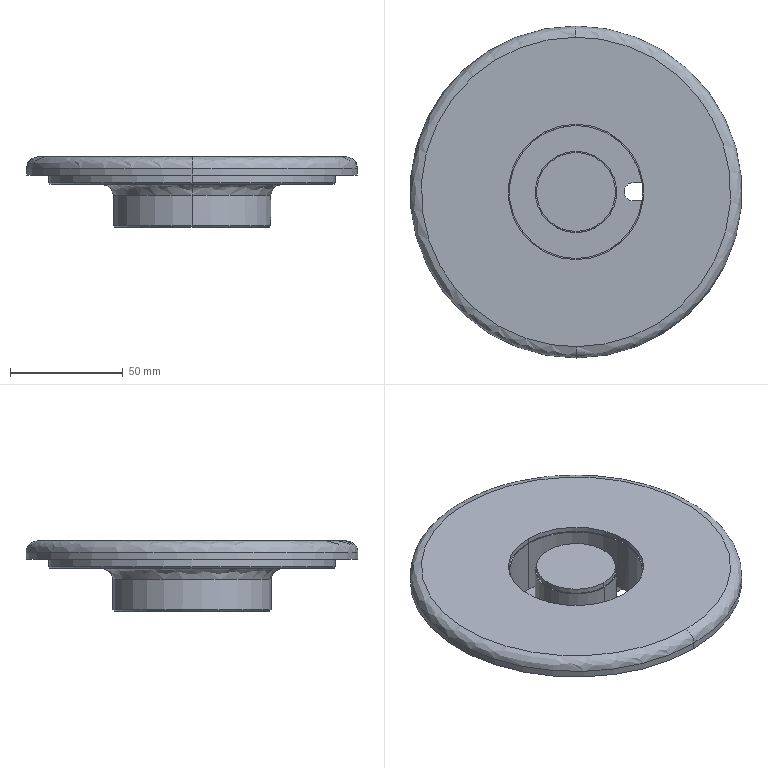Part | SolidWorks | features BaseBody 1 | 1 solid | 44 faces | box 147 x 147 x 31 mm | volume 210784 mm3 | cylinder 16 | cone 13 | plane 11 | spline 4 | commonest cylinder face diameters 8 x2 35 x2 36 x2 59 x2 60 x2 70 x2